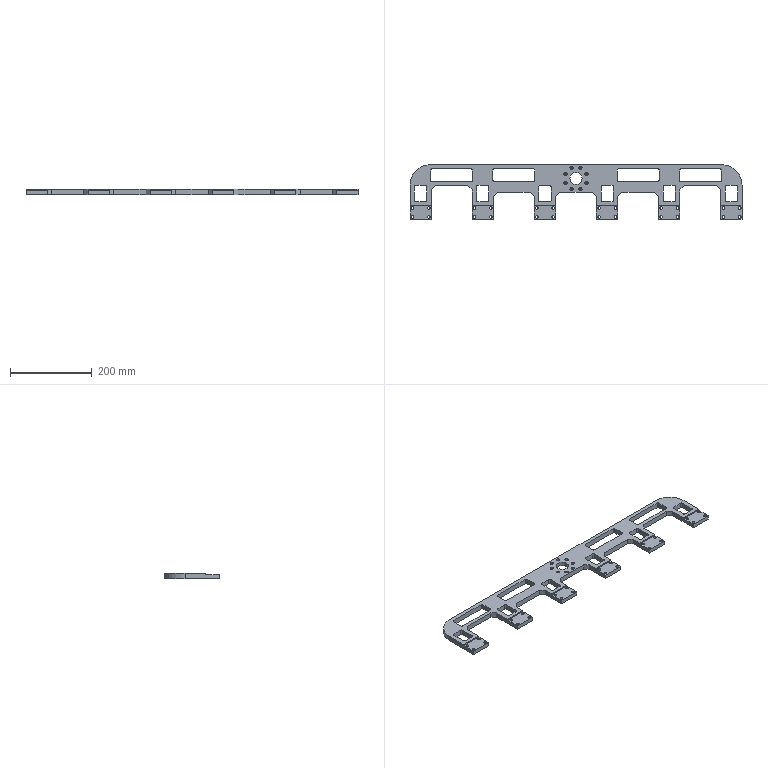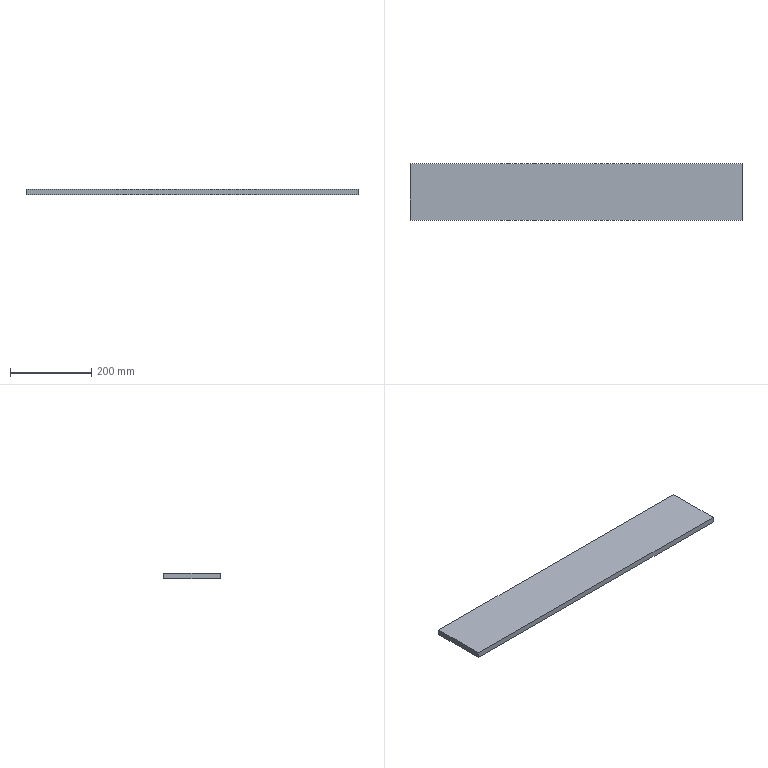CAM job | NX | 3-axis milling, drilling | part box 813.6 x 134 x 13 mm | stock box 817.6 x 138 x 14 mm
Tools:
number,name,description,diameter,corner_radius,flute_length,length,flutes
1,D63,Milling Tool-5 Parameters,63.0,0.0,50.0,75.0,2
7,D6A45,Milling Tool-5 Parameters,6.0,0.0,50.0,75.0,2
14,4.5ZT,Drilling Tool,4.5,0.0,35.0,50.0,2
15,6.5ZT,Drilling Tool,6.5,0.0,35.0,50.0,2
10,D10,Milling Tool-5 Parameters,10.0,0.0,50.0,75.0,2
6,D6,Milling Tool-5 Parameters,6.0,0.0,50.0,75.0,2
Operations:
program,operation,operation_type,tool,method,geometry_group,spindle_rpm,surface_speed,feed_per_tooth,feed_cut,feed_plunge,cut_length_mm,path_length_mm,cut_time_min,machine_time_min
1,FLOOR_WALL_COPY,VolumeBased25DMillingOperation,D63,METHOD,A,6500.0,1286.0,0.1154,1500.0,100.0,4527.797,4581.797,3.018,3.024
1,DRILLING_COPY_1,Operation,D6A45,METHOD,A,5000.0,94.0,0.025,250.0,0.0,132.0,1695.158,0.528,0.6843
1,DRILLING_COPY_COPY_1,Operation,4.5ZT,METHOD,A,2000.0,28.0,0.0625,250.0,0.0,146.815,526.106,0.5873,0.6252
1,DRILLING_COPY_COPY_COPY,Operation,6.5ZT,METHOD,A,2000.0,28.0,0.0625,250.0,0.0,454.867,2108.052,1.819,1.985
1,ZLEVEL_PROFILE_COPY_3,ZLevelMilling,D10,METHOD,A,9500.0,298.0,0.1842,3500.0,1000.0,33196.656,33266.056,9.518,9.525
1,ZLEVEL_PROFILE_COPY_2_COPY,ZLevelMilling,D10,METHOD,A,9500.0,298.0,0.1842,3500.0,1000.0,21517.198,23772.992,6.522,6.747
1,ZLEVEL_PROFILE_COPY_COPY_1,ZLevelMilling,D10,METHOD,A,9500.0,298.0,0.0789,1500.0,1000.0,6253.482,8621.69,4.281,4.518
1,FLOOR_WALL_1_COPY_1,VolumeBased25DMillingOperation,D10,METHOD,A,9500.0,298.0,0.1579,3000.0,1000.0,9231.884,10587.304,3.122,3.257
1,FLOOR_WALL_1_COPY_COPY,VolumeBased25DMillingOperation,D10,METHOD,A,9500.0,298.0,0.0789,1500.0,1000.0,2517.148,3732.593,1.7,2.038
1,HOLE_MILLING_COPY,CylinderMilling,D6,METHOD,A,9500.0,179.0,0.0737,1400.0,100.0,589.727,1252.539,0.4212,0.4875
1,ZLEVEL_PROFILE_COPY_1_COPY,ZLevelMilling,D6,METHOD,A,9500.0,179.0,0.0868,1650.0,1000.0,6115.821,13413.548,4.143,4.873
1,PLANAR_MILL_COPY_1,PlanarMilling,D6A45,METHOD,A,9500.0,179.0,0.0737,1400.0,100.0,4282.417,6719.428,3.059,3.303
1,PLANAR_MILL_COPY_1_COPY,PlanarMilling,D6A45,METHOD,A,9500.0,179.0,0.0737,1400.0,100.0,1199.731,5674.415,0.857,1.304
1,ZLEVEL_PROFILE_COPY_3_COPY,ZLevelMilling,D10,METHOD,A,9500.0,298.0,0.0632,1200.0,1000.0,10206.578,10282.003,8.507,8.515
2,FLOOR_WALL_COPY_COPY,VolumeBased25DMillingOperation,D63,METHOD,B,6500.0,1286.0,0.1154,1500.0,100.0,4527.797,4581.797,3.018,3.024
2,DRILLING_COPY_1_COPY,Operation,D6A45,METHOD,B,5000.0,94.0,0.025,250.0,0.0,132.0,1697.29,0.528,0.6845
2,DRILLING_COPY_COPY_1_COPY,Operation,4.5ZT,METHOD,B,2000.0,28.0,0.0625,250.0,0.0,146.815,526.106,0.5873,0.6252
2,DRILLING_COPY_COPY_COPY_COPY,Operation,6.5ZT,METHOD,B,2000.0,28.0,0.0625,250.0,0.0,454.867,2108.052,1.819,1.985
2,ZLEVEL_PROFILE_COPY_3_COPY_1,ZLevelMilling,D10,METHOD,B,9500.0,298.0,0.1842,3500.0,1000.0,33196.656,33266.056,9.518,9.525
2,HOLE_MILLING,CylinderMilling,D10,METHOD,B,8500.0,267.0,0.1176,2000.0,100.0,2401.112,2463.112,1.201,1.207
2,FLOOR_WALL_1_COPY_COPY_COPY,VolumeBased25DMillingOperation,D10,METHOD,B,9500.0,298.0,0.0789,1500.0,1000.0,627.575,713.856,0.4202,0.4556
2,ZLEVEL_PROFILE_COPY_2_COPY_COPY,ZLevelMilling,D10,METHOD,B,9500.0,298.0,0.1842,3500.0,1000.0,21517.195,23781.062,6.522,6.748
2,ZLEVEL_PROFILE_COPY_COPY_1_COPY,ZLevelMilling,D10,METHOD,B,9500.0,298.0,0.0789,1500.0,1000.0,6253.468,8547.432,4.281,4.51
2,PLANAR_MILL_COPY_1_COPY_1,PlanarMilling,D6A45,METHOD,B,9500.0,179.0,0.0737,1400.0,100.0,5080.462,8991.976,3.629,4.02
2,PLANAR_MILL_COPY_1_COPY_1_COPY,PlanarMilling,D6A45,METHOD,B,9500.0,179.0,0.0737,1400.0,100.0,94.458,160.458,0.0675,0.0741